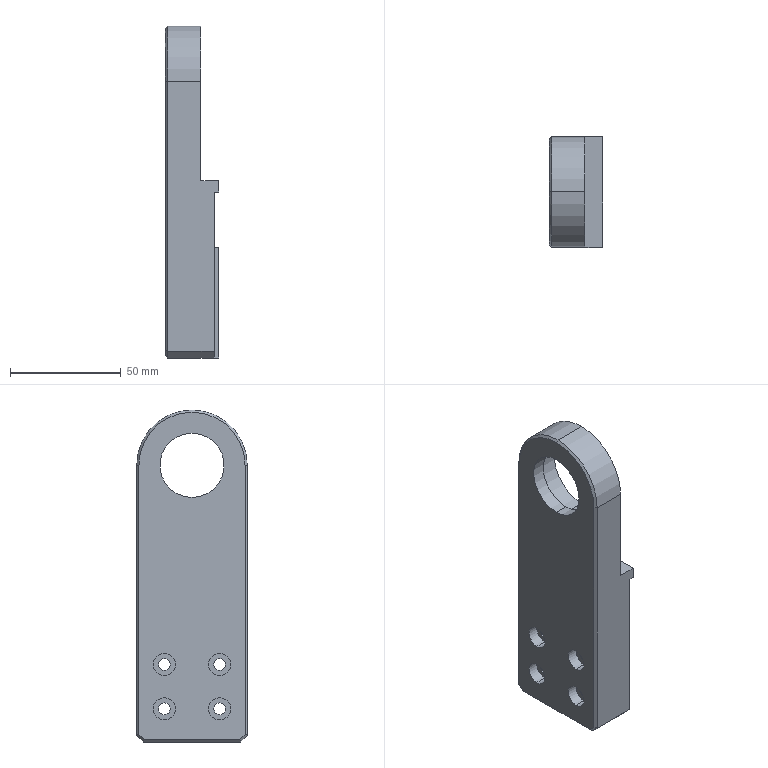Part | STEP file | CON-001 | 1 solid | 53 faces | box 24 x 50 x 150 mm | volume 124182 mm3 | plane 29 | cylinder 22 | cone 2 | commonest cylinder face diameters 5.3 x8 10 x8 29 x2 35 x2 50 x2